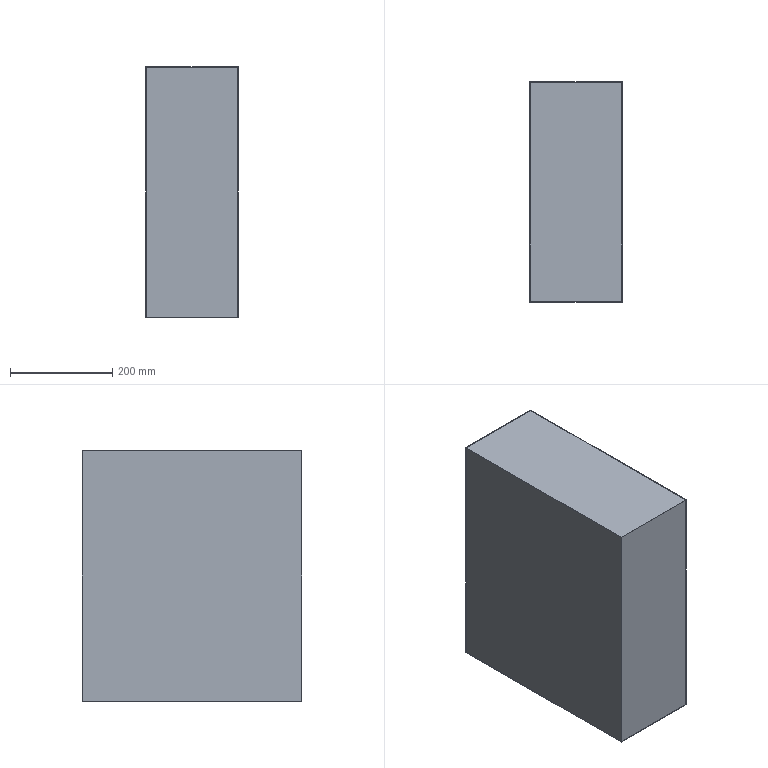Part | STEP file | yh610h | 1 solid | 11 faces | box 180 x 430 x 490 mm | volume 672024 mm3 | plane 11
STEP:
#1=CARTESIAN_POINT('',(-3242.97,-5486.461,-480.));
#2=VERTEX_POINT('',#1);
#3=CARTESIAN_POINT('',(-3242.97,-5486.461,10.));
#4=VERTEX_POINT('',#3);
#5=CARTESIAN_POINT('',(-3242.97,-5486.461,-480.));
#6=DIRECTION('',(0.,0.,1.));
#7=VECTOR('',#6,1000.);
#8=LINE('',#5,#7);
#9=EDGE_CURVE('',#2,#4,#8,.T.);
#10=ORIENTED_EDGE('',*,*,#9,.T.);
#11=CARTESIAN_POINT('',(-3242.97,-5056.461,10.));
#12=VERTEX_POINT('',#11);
#13=CARTESIAN_POINT('',(-3242.97,-5056.461,10.));
#14=DIRECTION('',(0.,-1.,0.));
#15=VECTOR('',#14,1000.);
#16=LINE('',#13,#15);
#17=EDGE_CURVE('',#12,#4,#16,.T.);
#18=ORIENTED_EDGE('',*,*,#17,.F.);
#19=CARTESIAN_POINT('',(-3242.97,-5056.461,-480.));
#20=VERTEX_POINT('',#19);
#21=CARTESIAN_POINT('',(-3242.97,-5056.461,-480.));
#22=DIRECTION('',(0.,0.,1.));
#23=VECTOR('',#22,1000.);
#24=LINE('',#21,#23);
#25=EDGE_CURVE('',#20,#12,#24,.T.);
#26=ORIENTED_EDGE('',*,*,#25,.F.);
#27=CARTESIAN_POINT('',(-3242.97,-5056.461,-480.));
#28=DIRECTION('',(0.,-1.,0.));
#29=VECTOR('',#28,1000.);
#30=LINE('',#27,#29);
#31=EDGE_CURVE('',#20,#2,#30,.T.);
#32=ORIENTED_EDGE('',*,*,#31,.T.);
#33=EDGE_LOOP('',(#10,#18,#26,#32));
#34=FACE_OUTER_BOUND('',#33,.T.);
#35=CARTESIAN_POINT('',(-3242.97,-5056.461,-480.));
#36=DIRECTION('',(-1.,0.,0.));
#37=DIRECTION('',(0.,-1.,0.));
#38=AXIS2_PLACEMENT_3D('',#35,#36,#37);
#39=PLANE('',#38);
#40=ADVANCED_FACE('',(#34),#39,.T.);
#41=ORIENTED_EDGE('',*,*,#25,.T.);
#42=CARTESIAN_POINT('',(-3062.97,-5056.461,10.));
#43=VERTEX_POINT('',#42);
#44=CARTESIAN_POINT('',(-3242.97,-5056.461,10.));
#45=DIRECTION('',(-1.,0.,0.));
#46=VECTOR('',#45,1000.);
#47=LINE('',#44,#46);
#48=EDGE_CURVE('',#43,#12,#47,.T.);
#49=ORIENTED_EDGE('',*,*,#48,.F.);
#50=CARTESIAN_POINT('',(-3062.97,-5056.461,-480.));
#51=VERTEX_POINT('',#50);
#52=CARTESIAN_POINT('',(-3062.97,-5056.461,-480.));
#53=DIRECTION('',(0.,0.,1.));
#54=VECTOR('',#53,1000.);
#55=LINE('',#52,#54);
#56=EDGE_CURVE('',#51,#43,#55,.T.);
#57=ORIENTED_EDGE('',*,*,#56,.F.);
#58=CARTESIAN_POINT('',(-3242.97,-5056.461,-480.));
#59=DIRECTION('',(-1.,0.,0.));
#60=VECTOR('',#59,1000.);
#61=LINE('',#58,#60);
#62=EDGE_CURVE('',#51,#20,#61,.T.);
#63=ORIENTED_EDGE('',*,*,#62,.T.);
#64=EDGE_LOOP('',(#41,#49,#57,#63));
#65=FACE_OUTER_BOUND('',#64,.T.);
#66=CARTESIAN_POINT('',(-3242.97,-5056.461,-480.));
#67=DIRECTION('',(0.,1.,0.));
#68=DIRECTION('',(0.,0.,1.));
#69=AXIS2_PLACEMENT_3D('',#66,#67,#68);
#70=PLANE('',#69);
#71=ADVANCED_FACE('',(#65),#70,.T.);
#72=ORIENTED_EDGE('',*,*,#56,.T.);
#73=CARTESIAN_POINT('',(-3062.97,-5486.461,10.));
#74=VERTEX_POINT('',#73);
#75=CARTESIAN_POINT('',(-3062.97,-5056.461,10.));
#76=DIRECTION('',(0.,1.,0.));
#77=VECTOR('',#76,1000.);
#78=LINE('',#75,#77);
#79=EDGE_CURVE('',#74,#43,#78,.T.);
#80=ORIENTED_EDGE('',*,*,#79,.F.);
#81=CARTESIAN_POINT('',(-3062.97,-5486.461,-480.));
#82=VERTEX_POINT('',#81);
#83=CARTESIAN_POINT('',(-3062.97,-5486.461,-480.));
#84=DIRECTION('',(0.,0.,1.));
#85=VECTOR('',#84,1000.);
#86=LINE('',#83,#85);
#87=EDGE_CURVE('',#82,#74,#86,.T.);
#88=ORIENTED_EDGE('',*,*,#87,.F.);
#89=CARTESIAN_POINT('',(-3062.97,-5056.461,-480.));
#90=DIRECTION('',(0.,1.,0.));
#91=VECTOR('',#90,1000.);
#92=LINE('',#89,#91);
#93=EDGE_CURVE('',#82,#51,#92,.T.);
#94=ORIENTED_EDGE('',*,*,#93,.T.);
#95=EDGE_LOOP('',(#72,#80,#88,#94));
#96=FACE_OUTER_BOUND('',#95,.T.);
#97=CARTESIAN_POINT('',(-3062.97,-5056.461,-480.));
#98=DIRECTION('',(1.,0.,0.));
#99=DIRECTION('',(0.,0.,-1.));
#100=AXIS2_PLACEMENT_3D('',#97,#98,#99);
#101=PLANE('',#100);
#102=ADVANCED_FACE('',(#96),#101,.T.);
#103=ORIENTED_EDGE('',*,*,#87,.T.);
#104=CARTESIAN_POINT('',(-3242.97,-5486.461,10.));
#105=DIRECTION('',(1.,0.,0.));
#106=VECTOR('',#105,1000.);
#107=LINE('',#104,#106);
#108=EDGE_CURVE('',#4,#74,#107,.T.);
#109=ORIENTED_EDGE('',*,*,#108,.F.);
#110=ORIENTED_EDGE('',*,*,#9,.F.);
#111=CARTESIAN_POINT('',(-3242.97,-5486.461,-480.));
#112=DIRECTION('',(1.,0.,0.));
#113=VECTOR('',#112,1000.);
#114=LINE('',#111,#113);
#115=EDGE_CURVE('',#2,#82,#114,.T.);
#116=ORIENTED_EDGE('',*,*,#115,.T.);
#117=EDGE_LOOP('',(#103,#109,#110,#116));
#118=FACE_OUTER_BOUND('',#117,.T.);
#119=CARTESIAN_POINT('',(-3242.97,-5486.461,-480.));
#120=DIRECTION('',(0.,-1.,0.));
#121=DIRECTION('',(0.,0.,-1.));
#122=AXIS2_PLACEMENT_3D('',#119,#120,#121);
#123=PLANE('',#122);
#124=ADVANCED_FACE('',(#118),#123,.T.);
#125=CARTESIAN_POINT('',(-3063.97,-5057.461,-480.));
#126=VERTEX_POINT('',#125);
#127=CARTESIAN_POINT('',(-3241.97,-5057.461,-480.));
#128=VERTEX_POINT('',#127);
#129=CARTESIAN_POINT('',(-3242.97,-5057.461,-480.));
#130=DIRECTION('',(-1.,0.,0.));
#131=VECTOR('',#130,1000.);
#132=LINE('',#129,#131);
#133=EDGE_CURVE('',#126,#128,#132,.T.);
#134=ORIENTED_EDGE('',*,*,#133,.T.);
#135=CARTESIAN_POINT('',(-3241.97,-5485.461,-480.));
#136=VERTEX_POINT('',#135);
#137=CARTESIAN_POINT('',(-3241.97,-5486.461,-480.));
#138=DIRECTION('',(0.,-1.,0.));
#139=VECTOR('',#138,1000.);
#140=LINE('',#137,#139);
#141=EDGE_CURVE('',#128,#136,#140,.T.);
#142=ORIENTED_EDGE('',*,*,#141,.T.);
#143=CARTESIAN_POINT('',(-3063.97,-5485.461,-480.));
#144=VERTEX_POINT('',#143);
#145=CARTESIAN_POINT('',(-3242.97,-5485.461,-480.));
#146=DIRECTION('',(1.,0.,0.));
#147=VECTOR('',#146,1000.);
#148=LINE('',#145,#147);
#149=EDGE_CURVE('',#136,#144,#148,.T.);
#150=ORIENTED_EDGE('',*,*,#149,.T.);
#151=CARTESIAN_POINT('',(-3063.97,-5486.461,-480.));
#152=DIRECTION('',(0.,1.,0.));
#153=VECTOR('',#152,1000.);
#154=LINE('',#151,#153);
#155=EDGE_CURVE('',#144,#126,#154,.T.);
#156=ORIENTED_EDGE('',*,*,#155,.T.);
#157=EDGE_LOOP('',(#134,#142,#150,#156));
#158=FACE_BOUND('',#157,.T.);
#159=ORIENTED_EDGE('',*,*,#31,.F.);
#160=ORIENTED_EDGE('',*,*,#62,.F.);
#161=ORIENTED_EDGE('',*,*,#93,.F.);
#162=ORIENTED_EDGE('',*,*,#115,.F.);
#163=EDGE_LOOP('',(#159,#160,#161,#162));
#164=FACE_OUTER_BOUND('',#163,.T.);
#165=CARTESIAN_POINT('',(-3242.97,-5486.461,-480.));
#166=DIRECTION('',(0.,0.,1.));
#167=DIRECTION('',(1.,0.,0.));
#168=AXIS2_PLACEMENT_3D('',#165,#166,#167);
#169=PLANE('',#168);
#170=ADVANCED_FACE('',(#158,#164),#169,.F.);
#171=ORIENTED_EDGE('',*,*,#17,.T.);
#172=ORIENTED_EDGE('',*,*,#108,.T.);
#173=ORIENTED_EDGE('',*,*,#79,.T.);
#174=ORIENTED_EDGE('',*,*,#48,.T.);
#175=EDGE_LOOP('',(#171,#172,#173,#174));
#176=FACE_OUTER_BOUND('',#175,.T.);
#177=CARTESIAN_POINT('',(-3242.97,-5486.461,10.));
#178=DIRECTION('',(0.,0.,1.));
#179=DIRECTION('',(1.,0.,0.));
#180=AXIS2_PLACEMENT_3D('',#177,#178,#179);
#181=PLANE('',#180);
#182=ADVANCED_FACE('',(#176),#181,.T.);
#183=CARTESIAN_POINT('',(-3241.97,-5485.461,9.));
#184=VERTEX_POINT('',#183);
#185=CARTESIAN_POINT('',(-3241.97,-5485.461,-480.));
#186=DIRECTION('',(0.,0.,1.));
#187=VECTOR('',#186,1000.);
#188=LINE('',#185,#187);
#189=EDGE_CURVE('',#136,#184,#188,.T.);
#190=ORIENTED_EDGE('',*,*,#189,.F.);
#191=ORIENTED_EDGE('',*,*,#141,.F.);
#192=CARTESIAN_POINT('',(-3241.97,-5057.461,9.));
#193=VERTEX_POINT('',#192);
#194=CARTESIAN_POINT('',(-3241.97,-5057.461,-480.));
#195=DIRECTION('',(0.,0.,1.));
#196=VECTOR('',#195,1000.);
#197=LINE('',#194,#196);
#198=EDGE_CURVE('',#128,#193,#197,.T.);
#199=ORIENTED_EDGE('',*,*,#198,.T.);
#200=CARTESIAN_POINT('',(-3241.97,-5486.461,9.));
#201=DIRECTION('',(0.,-1.,0.));
#202=VECTOR('',#201,1000.);
#203=LINE('',#200,#202);
#204=EDGE_CURVE('',#193,#184,#203,.T.);
#205=ORIENTED_EDGE('',*,*,#204,.T.);
#206=EDGE_LOOP('',(#190,#191,#199,#205));
#207=FACE_OUTER_BOUND('',#206,.T.);
#208=CARTESIAN_POINT('',(-3241.97,-5056.461,-480.));
#209=DIRECTION('',(-1.,0.,0.));
#210=DIRECTION('',(0.,-1.,0.));
#211=AXIS2_PLACEMENT_3D('',#208,#209,#210);
#212=PLANE('',#211);
#213=ADVANCED_FACE('',(#207),#212,.F.);
#214=ORIENTED_EDGE('',*,*,#198,.F.);
#215=ORIENTED_EDGE('',*,*,#133,.F.);
#216=CARTESIAN_POINT('',(-3063.97,-5057.461,9.));
#217=VERTEX_POINT('',#216);
#218=CARTESIAN_POINT('',(-3063.97,-5057.461,-480.));
#219=DIRECTION('',(0.,0.,1.));
#220=VECTOR('',#219,1000.);
#221=LINE('',#218,#220);
#222=EDGE_CURVE('',#126,#217,#221,.T.);
#223=ORIENTED_EDGE('',*,*,#222,.T.);
#224=CARTESIAN_POINT('',(-3242.97,-5057.461,9.));
#225=DIRECTION('',(-1.,0.,0.));
#226=VECTOR('',#225,1000.);
#227=LINE('',#224,#226);
#228=EDGE_CURVE('',#217,#193,#227,.T.);
#229=ORIENTED_EDGE('',*,*,#228,.T.);
#230=EDGE_LOOP('',(#214,#215,#223,#229));
#231=FACE_OUTER_BOUND('',#230,.T.);
#232=CARTESIAN_POINT('',(-3242.97,-5057.461,-480.));
#233=DIRECTION('',(0.,1.,0.));
#234=DIRECTION('',(0.,0.,1.));
#235=AXIS2_PLACEMENT_3D('',#232,#233,#234);
#236=PLANE('',#235);
#237=ADVANCED_FACE('',(#231),#236,.F.);
#238=ORIENTED_EDGE('',*,*,#222,.F.);
#239=ORIENTED_EDGE('',*,*,#155,.F.);
#240=CARTESIAN_POINT('',(-3063.97,-5485.461,9.));
#241=VERTEX_POINT('',#240);
#242=CARTESIAN_POINT('',(-3063.97,-5485.461,-480.));
#243=DIRECTION('',(0.,0.,1.));
#244=VECTOR('',#243,1000.);
#245=LINE('',#242,#244);
#246=EDGE_CURVE('',#144,#241,#245,.T.);
#247=ORIENTED_EDGE('',*,*,#246,.T.);
#248=CARTESIAN_POINT('',(-3063.97,-5486.461,9.));
#249=DIRECTION('',(0.,1.,0.));
#250=VECTOR('',#249,1000.);
#251=LINE('',#248,#250);
#252=EDGE_CURVE('',#241,#217,#251,.T.);
#253=ORIENTED_EDGE('',*,*,#252,.T.);
#254=EDGE_LOOP('',(#238,#239,#247,#253));
#255=FACE_OUTER_BOUND('',#254,.T.);
#256=CARTESIAN_POINT('',(-3063.97,-5056.461,-480.));
#257=DIRECTION('',(1.,0.,0.));
#258=DIRECTION('',(0.,0.,-1.));
#259=AXIS2_PLACEMENT_3D('',#256,#257,#258);
#260=PLANE('',#259);
#261=ADVANCED_FACE('',(#255),#260,.F.);
#262=ORIENTED_EDGE('',*,*,#246,.F.);
#263=ORIENTED_EDGE('',*,*,#149,.F.);
#264=ORIENTED_EDGE('',*,*,#189,.T.);
#265=CARTESIAN_POINT('',(-3242.97,-5485.461,9.));
#266=DIRECTION('',(1.,0.,0.));
#267=VECTOR('',#266,1000.);
#268=LINE('',#265,#267);
#269=EDGE_CURVE('',#184,#241,#268,.T.);
#270=ORIENTED_EDGE('',*,*,#269,.T.);
#271=EDGE_LOOP('',(#262,#263,#264,#270));
#272=FACE_OUTER_BOUND('',#271,.T.);
#273=CARTESIAN_POINT('',(-3242.97,-5485.461,-480.));
#274=DIRECTION('',(0.,-1.,0.));
#275=DIRECTION('',(0.,0.,-1.));
#276=AXIS2_PLACEMENT_3D('',#273,#274,#275);
#277=PLANE('',#276);
#278=ADVANCED_FACE('',(#272),#277,.F.);
#279=ORIENTED_EDGE('',*,*,#204,.F.);
#280=ORIENTED_EDGE('',*,*,#228,.F.);
#281=ORIENTED_EDGE('',*,*,#252,.F.);
#282=ORIENTED_EDGE('',*,*,#269,.F.);
#283=EDGE_LOOP('',(#279,#280,#281,#282));
#284=FACE_OUTER_BOUND('',#283,.T.);
#285=CARTESIAN_POINT('',(-3242.97,-5486.461,9.));
#286=DIRECTION('',(0.,0.,1.));
#287=DIRECTION('',(1.,0.,0.));
#288=AXIS2_PLACEMENT_3D('',#285,#286,#287);
#289=PLANE('',#288);
#290=ADVANCED_FACE('',(#284),#289,.F.);
#291=CLOSED_SHELL('',(#40,#71,#102,#124,#170,#182,#213,#237,#261,#278,#290));
#292=MANIFOLD_SOLID_BREP('',#291);
#293=CARTESIAN_POINT('',(0.,0.,0.));
#294=DIRECTION('',(0.,0.,1.));
#295=DIRECTION('',(1.,0.,0.));
#296=AXIS2_PLACEMENT_3D('',#293,#294,#295);
#297=(LENGTH_UNIT()NAMED_UNIT(*)SI_UNIT(.MILLI.,.METRE.));
#298=UNCERTAINTY_MEASURE_WITH_UNIT(LENGTH_MEASURE(0.00001),#297,'','');
#299=(NAMED_UNIT(*)PLANE_ANGLE_UNIT()SI_UNIT($,.RADIAN.));
#300=(NAMED_UNIT(*)SI_UNIT($,.STERADIAN.)SOLID_ANGLE_UNIT());
#301=(GEOMETRIC_REPRESENTATION_CONTEXT(3)GLOBAL_UNCERTAINTY_ASSIGNED_CONTEXT((#298))GLOBAL_UNIT_ASSIGNED_CONTEXT((#297,#299,#300))REPRESENTATION_CONTEXT('',''));
#302=ADVANCED_BREP_SHAPE_REPRESENTATION('',(#292,#296),#301);